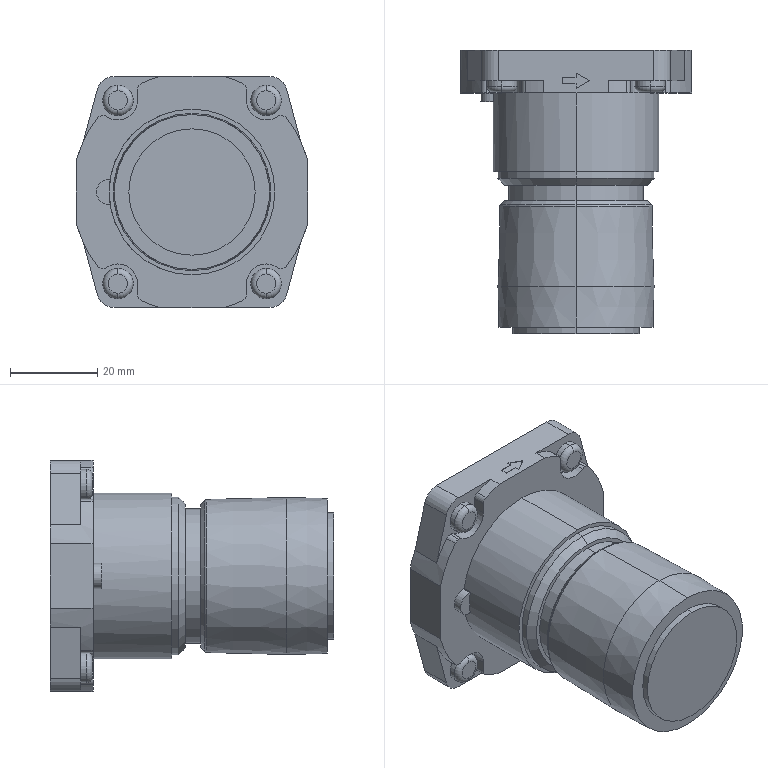Part | SolidWorks | features BaseBody 1 | 1 solid | 109 faces | box 53 x 65 x 53 mm | volume 80542 mm3 | cylinder 47 | plane 44 | torus 10 | cone 8 | commonest cylinder face diameters 3 x10 7 x8 55 x8 9 x6 8 x4 5.8 x3